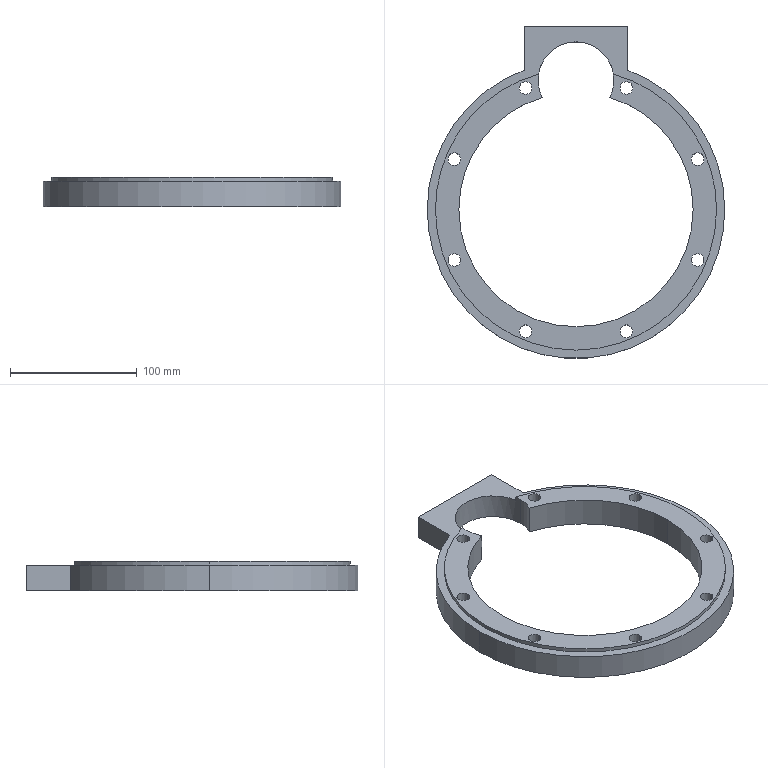Part | SolidWorks | features ICE 2, Cut 1, Extrusion 1, HoleWzd 1 | 1 solid | 34 faces | box 235 x 262.5 x 23 mm | volume 355148 mm3 | cylinder 28 | plane 6 | commonest cylinder face diameters 10 x16 60 x3 185 x3 222 x3 235 x3
STEP:
#1=CARTESIAN_POINT('',(44.799,96.083,23.));
#2=VERTEX_POINT('',#1);
#3=CARTESIAN_POINT('',(34.799,96.083,23.));
#4=VERTEX_POINT('',#3);
#5=CARTESIAN_POINT('',(39.799,96.083,23.));
#6=DIRECTION('',(0.,0.,-1.));
#7=DIRECTION('',(-1.,0.,0.));
#8=AXIS2_PLACEMENT_3D('',#5,#6,#7);
#9=CIRCLE('',#8,5.);
#10=EDGE_CURVE('',#2,#4,#9,.T.);
#11=ORIENTED_EDGE('',*,*,#10,.F.);
#12=CARTESIAN_POINT('',(44.799,96.083,0.));
#13=VERTEX_POINT('',#12);
#14=CARTESIAN_POINT('',(44.799,96.083,0.));
#15=DIRECTION('',(0.,0.,-1.));
#16=VECTOR('',#15,1000.);
#17=LINE('',#14,#16);
#18=EDGE_CURVE('',#2,#13,#17,.T.);
#19=ORIENTED_EDGE('',*,*,#18,.T.);
#20=CARTESIAN_POINT('',(34.799,96.083,0.));
#21=VERTEX_POINT('',#20);
#22=CARTESIAN_POINT('',(39.799,96.083,0.));
#23=DIRECTION('',(0.,0.,-1.));
#24=DIRECTION('',(-1.,0.,0.));
#25=AXIS2_PLACEMENT_3D('',#22,#23,#24);
#26=CIRCLE('',#25,5.);
#27=EDGE_CURVE('',#13,#21,#26,.T.);
#28=ORIENTED_EDGE('',*,*,#27,.T.);
#29=CARTESIAN_POINT('',(34.799,96.083,0.));
#30=DIRECTION('',(0.,0.,-1.));
#31=VECTOR('',#30,1000.);
#32=LINE('',#29,#31);
#33=EDGE_CURVE('',#4,#21,#32,.T.);
#34=ORIENTED_EDGE('',*,*,#33,.F.);
#35=EDGE_LOOP('',(#11,#19,#28,#34));
#36=FACE_OUTER_BOUND('',#35,.T.);
#37=CARTESIAN_POINT('',(39.799,96.083,0.));
#38=DIRECTION('',(0.,0.,-1.));
#39=DIRECTION('',(-1.,0.,0.));
#40=AXIS2_PLACEMENT_3D('',#37,#38,#39);
#41=CYLINDRICAL_SURFACE('',#40,5.);
#42=ADVANCED_FACE('',(#36),#41,.F.);
#43=CARTESIAN_POINT('',(101.083,39.799,23.));
#44=VERTEX_POINT('',#43);
#45=CARTESIAN_POINT('',(91.083,39.799,23.));
#46=VERTEX_POINT('',#45);
#47=CARTESIAN_POINT('',(96.083,39.799,23.));
#48=DIRECTION('',(0.,0.,-1.));
#49=DIRECTION('',(-1.,0.,0.));
#50=AXIS2_PLACEMENT_3D('',#47,#48,#49);
#51=CIRCLE('',#50,5.);
#52=EDGE_CURVE('',#44,#46,#51,.T.);
#53=ORIENTED_EDGE('',*,*,#52,.F.);
#54=CARTESIAN_POINT('',(101.083,39.799,0.));
#55=VERTEX_POINT('',#54);
#56=CARTESIAN_POINT('',(101.083,39.799,0.));
#57=DIRECTION('',(0.,0.,-1.));
#58=VECTOR('',#57,1000.);
#59=LINE('',#56,#58);
#60=EDGE_CURVE('',#44,#55,#59,.T.);
#61=ORIENTED_EDGE('',*,*,#60,.T.);
#62=CARTESIAN_POINT('',(91.083,39.799,0.));
#63=VERTEX_POINT('',#62);
#64=CARTESIAN_POINT('',(96.083,39.799,0.));
#65=DIRECTION('',(0.,0.,-1.));
#66=DIRECTION('',(-1.,0.,0.));
#67=AXIS2_PLACEMENT_3D('',#64,#65,#66);
#68=CIRCLE('',#67,5.);
#69=EDGE_CURVE('',#55,#63,#68,.T.);
#70=ORIENTED_EDGE('',*,*,#69,.T.);
#71=CARTESIAN_POINT('',(91.083,39.799,0.));
#72=DIRECTION('',(0.,0.,-1.));
#73=VECTOR('',#72,1000.);
#74=LINE('',#71,#73);
#75=EDGE_CURVE('',#46,#63,#74,.T.);
#76=ORIENTED_EDGE('',*,*,#75,.F.);
#77=EDGE_LOOP('',(#53,#61,#70,#76));
#78=FACE_OUTER_BOUND('',#77,.T.);
#79=CARTESIAN_POINT('',(96.083,39.799,0.));
#80=DIRECTION('',(0.,0.,-1.));
#81=DIRECTION('',(-1.,0.,0.));
#82=AXIS2_PLACEMENT_3D('',#79,#80,#81);
#83=CYLINDRICAL_SURFACE('',#82,5.);
#84=ADVANCED_FACE('',(#78),#83,.F.);
#85=CARTESIAN_POINT('',(101.083,-39.799,23.));
#86=VERTEX_POINT('',#85);
#87=CARTESIAN_POINT('',(91.083,-39.799,23.));
#88=VERTEX_POINT('',#87);
#89=CARTESIAN_POINT('',(96.083,-39.799,23.));
#90=DIRECTION('',(0.,0.,-1.));
#91=DIRECTION('',(-1.,0.,0.));
#92=AXIS2_PLACEMENT_3D('',#89,#90,#91);
#93=CIRCLE('',#92,5.);
#94=EDGE_CURVE('',#86,#88,#93,.T.);
#95=ORIENTED_EDGE('',*,*,#94,.F.);
#96=CARTESIAN_POINT('',(101.083,-39.799,0.));
#97=VERTEX_POINT('',#96);
#98=CARTESIAN_POINT('',(101.083,-39.799,0.));
#99=DIRECTION('',(0.,0.,-1.));
#100=VECTOR('',#99,1000.);
#101=LINE('',#98,#100);
#102=EDGE_CURVE('',#86,#97,#101,.T.);
#103=ORIENTED_EDGE('',*,*,#102,.T.);
#104=CARTESIAN_POINT('',(91.083,-39.799,0.));
#105=VERTEX_POINT('',#104);
#106=CARTESIAN_POINT('',(96.083,-39.799,0.));
#107=DIRECTION('',(0.,0.,-1.));
#108=DIRECTION('',(-1.,0.,0.));
#109=AXIS2_PLACEMENT_3D('',#106,#107,#108);
#110=CIRCLE('',#109,5.);
#111=EDGE_CURVE('',#97,#105,#110,.T.);
#112=ORIENTED_EDGE('',*,*,#111,.T.);
#113=CARTESIAN_POINT('',(91.083,-39.799,0.));
#114=DIRECTION('',(0.,0.,-1.));
#115=VECTOR('',#114,1000.);
#116=LINE('',#113,#115);
#117=EDGE_CURVE('',#88,#105,#116,.T.);
#118=ORIENTED_EDGE('',*,*,#117,.F.);
#119=EDGE_LOOP('',(#95,#103,#112,#118));
#120=FACE_OUTER_BOUND('',#119,.T.);
#121=CARTESIAN_POINT('',(96.083,-39.799,0.));
#122=DIRECTION('',(0.,0.,-1.));
#123=DIRECTION('',(-1.,0.,0.));
#124=AXIS2_PLACEMENT_3D('',#121,#122,#123);
#125=CYLINDRICAL_SURFACE('',#124,5.);
#126=ADVANCED_FACE('',(#120),#125,.F.);
#127=CARTESIAN_POINT('',(44.799,-96.083,23.));
#128=VERTEX_POINT('',#127);
#129=CARTESIAN_POINT('',(34.799,-96.083,23.));
#130=VERTEX_POINT('',#129);
#131=CARTESIAN_POINT('',(39.799,-96.083,23.));
#132=DIRECTION('',(0.,0.,-1.));
#133=DIRECTION('',(-1.,0.,0.));
#134=AXIS2_PLACEMENT_3D('',#131,#132,#133);
#135=CIRCLE('',#134,5.);
#136=EDGE_CURVE('',#128,#130,#135,.T.);
#137=ORIENTED_EDGE('',*,*,#136,.F.);
#138=CARTESIAN_POINT('',(44.799,-96.083,0.));
#139=VERTEX_POINT('',#138);
#140=CARTESIAN_POINT('',(44.799,-96.083,0.));
#141=DIRECTION('',(0.,0.,-1.));
#142=VECTOR('',#141,1000.);
#143=LINE('',#140,#142);
#144=EDGE_CURVE('',#128,#139,#143,.T.);
#145=ORIENTED_EDGE('',*,*,#144,.T.);
#146=CARTESIAN_POINT('',(34.799,-96.083,0.));
#147=VERTEX_POINT('',#146);
#148=CARTESIAN_POINT('',(39.799,-96.083,0.));
#149=DIRECTION('',(0.,0.,-1.));
#150=DIRECTION('',(-1.,0.,0.));
#151=AXIS2_PLACEMENT_3D('',#148,#149,#150);
#152=CIRCLE('',#151,5.);
#153=EDGE_CURVE('',#139,#147,#152,.T.);
#154=ORIENTED_EDGE('',*,*,#153,.T.);
#155=CARTESIAN_POINT('',(34.799,-96.083,0.));
#156=DIRECTION('',(0.,0.,-1.));
#157=VECTOR('',#156,1000.);
#158=LINE('',#155,#157);
#159=EDGE_CURVE('',#130,#147,#158,.T.);
#160=ORIENTED_EDGE('',*,*,#159,.F.);
#161=EDGE_LOOP('',(#137,#145,#154,#160));
#162=FACE_OUTER_BOUND('',#161,.T.);
#163=CARTESIAN_POINT('',(39.799,-96.083,0.));
#164=DIRECTION('',(0.,0.,-1.));
#165=DIRECTION('',(-1.,0.,0.));
#166=AXIS2_PLACEMENT_3D('',#163,#164,#165);
#167=CYLINDRICAL_SURFACE('',#166,5.);
#168=ADVANCED_FACE('',(#162),#167,.F.);
#169=CARTESIAN_POINT('',(-34.799,-96.083,23.));
#170=VERTEX_POINT('',#169);
#171=CARTESIAN_POINT('',(-44.799,-96.083,23.));
#172=VERTEX_POINT('',#171);
#173=CARTESIAN_POINT('',(-39.799,-96.083,23.));
#174=DIRECTION('',(0.,0.,-1.));
#175=DIRECTION('',(-1.,0.,0.));
#176=AXIS2_PLACEMENT_3D('',#173,#174,#175);
#177=CIRCLE('',#176,5.);
#178=EDGE_CURVE('',#170,#172,#177,.T.);
#179=ORIENTED_EDGE('',*,*,#178,.F.);
#180=CARTESIAN_POINT('',(-34.799,-96.083,0.));
#181=VERTEX_POINT('',#180);
#182=CARTESIAN_POINT('',(-34.799,-96.083,0.));
#183=DIRECTION('',(0.,0.,-1.));
#184=VECTOR('',#183,1000.);
#185=LINE('',#182,#184);
#186=EDGE_CURVE('',#170,#181,#185,.T.);
#187=ORIENTED_EDGE('',*,*,#186,.T.);
#188=CARTESIAN_POINT('',(-44.799,-96.083,0.));
#189=VERTEX_POINT('',#188);
#190=CARTESIAN_POINT('',(-39.799,-96.083,0.));
#191=DIRECTION('',(0.,0.,-1.));
#192=DIRECTION('',(-1.,0.,0.));
#193=AXIS2_PLACEMENT_3D('',#190,#191,#192);
#194=CIRCLE('',#193,5.);
#195=EDGE_CURVE('',#181,#189,#194,.T.);
#196=ORIENTED_EDGE('',*,*,#195,.T.);
#197=CARTESIAN_POINT('',(-44.799,-96.083,0.));
#198=DIRECTION('',(0.,0.,-1.));
#199=VECTOR('',#198,1000.);
#200=LINE('',#197,#199);
#201=EDGE_CURVE('',#172,#189,#200,.T.);
#202=ORIENTED_EDGE('',*,*,#201,.F.);
#203=EDGE_LOOP('',(#179,#187,#196,#202));
#204=FACE_OUTER_BOUND('',#203,.T.);
#205=CARTESIAN_POINT('',(-39.799,-96.083,0.));
#206=DIRECTION('',(0.,0.,-1.));
#207=DIRECTION('',(-1.,0.,0.));
#208=AXIS2_PLACEMENT_3D('',#205,#206,#207);
#209=CYLINDRICAL_SURFACE('',#208,5.);
#210=ADVANCED_FACE('',(#204),#209,.F.);
#211=CARTESIAN_POINT('',(-91.083,-39.799,23.));
#212=VERTEX_POINT('',#211);
#213=CARTESIAN_POINT('',(-101.083,-39.799,23.));
#214=VERTEX_POINT('',#213);
#215=CARTESIAN_POINT('',(-96.083,-39.799,23.));
#216=DIRECTION('',(0.,0.,-1.));
#217=DIRECTION('',(-1.,0.,0.));
#218=AXIS2_PLACEMENT_3D('',#215,#216,#217);
#219=CIRCLE('',#218,5.);
#220=EDGE_CURVE('',#212,#214,#219,.T.);
#221=ORIENTED_EDGE('',*,*,#220,.F.);
#222=CARTESIAN_POINT('',(-91.083,-39.799,0.));
#223=VERTEX_POINT('',#222);
#224=CARTESIAN_POINT('',(-91.083,-39.799,0.));
#225=DIRECTION('',(0.,0.,-1.));
#226=VECTOR('',#225,1000.);
#227=LINE('',#224,#226);
#228=EDGE_CURVE('',#212,#223,#227,.T.);
#229=ORIENTED_EDGE('',*,*,#228,.T.);
#230=CARTESIAN_POINT('',(-101.083,-39.799,0.));
#231=VERTEX_POINT('',#230);
#232=CARTESIAN_POINT('',(-96.083,-39.799,0.));
#233=DIRECTION('',(0.,0.,-1.));
#234=DIRECTION('',(-1.,0.,0.));
#235=AXIS2_PLACEMENT_3D('',#232,#233,#234);
#236=CIRCLE('',#235,5.);
#237=EDGE_CURVE('',#223,#231,#236,.T.);
#238=ORIENTED_EDGE('',*,*,#237,.T.);
#239=CARTESIAN_POINT('',(-101.083,-39.799,0.));
#240=DIRECTION('',(0.,0.,-1.));
#241=VECTOR('',#240,1000.);
#242=LINE('',#239,#241);
#243=EDGE_CURVE('',#214,#231,#242,.T.);
#244=ORIENTED_EDGE('',*,*,#243,.F.);
#245=EDGE_LOOP('',(#221,#229,#238,#244));
#246=FACE_OUTER_BOUND('',#245,.T.);
#247=CARTESIAN_POINT('',(-96.083,-39.799,0.));
#248=DIRECTION('',(0.,0.,-1.));
#249=DIRECTION('',(-1.,0.,0.));
#250=AXIS2_PLACEMENT_3D('',#247,#248,#249);
#251=CYLINDRICAL_SURFACE('',#250,5.);
#252=ADVANCED_FACE('',(#246),#251,.F.);
#253=CARTESIAN_POINT('',(-91.083,39.799,23.));
#254=VERTEX_POINT('',#253);
#255=CARTESIAN_POINT('',(-101.083,39.799,23.));
#256=VERTEX_POINT('',#255);
#257=CARTESIAN_POINT('',(-96.083,39.799,23.));
#258=DIRECTION('',(0.,0.,-1.));
#259=DIRECTION('',(-1.,0.,0.));
#260=AXIS2_PLACEMENT_3D('',#257,#258,#259);
#261=CIRCLE('',#260,5.);
#262=EDGE_CURVE('',#254,#256,#261,.T.);
#263=ORIENTED_EDGE('',*,*,#262,.F.);
#264=CARTESIAN_POINT('',(-91.083,39.799,0.));
#265=VERTEX_POINT('',#264);
#266=CARTESIAN_POINT('',(-91.083,39.799,0.));
#267=DIRECTION('',(0.,0.,-1.));
#268=VECTOR('',#267,1000.);
#269=LINE('',#266,#268);
#270=EDGE_CURVE('',#254,#265,#269,.T.);
#271=ORIENTED_EDGE('',*,*,#270,.T.);
#272=CARTESIAN_POINT('',(-101.083,39.799,0.));
#273=VERTEX_POINT('',#272);
#274=CARTESIAN_POINT('',(-96.083,39.799,0.));
#275=DIRECTION('',(0.,0.,-1.));
#276=DIRECTION('',(-1.,0.,0.));
#277=AXIS2_PLACEMENT_3D('',#274,#275,#276);
#278=CIRCLE('',#277,5.);
#279=EDGE_CURVE('',#265,#273,#278,.T.);
#280=ORIENTED_EDGE('',*,*,#279,.T.);
#281=CARTESIAN_POINT('',(-101.083,39.799,0.));
#282=DIRECTION('',(0.,0.,-1.));
#283=VECTOR('',#282,1000.);
#284=LINE('',#281,#283);
#285=EDGE_CURVE('',#256,#273,#284,.T.);
#286=ORIENTED_EDGE('',*,*,#285,.F.);
#287=EDGE_LOOP('',(#263,#271,#280,#286));
#288=FACE_OUTER_BOUND('',#287,.T.);
#289=CARTESIAN_POINT('',(-96.083,39.799,0.));
#290=DIRECTION('',(0.,0.,-1.));
#291=DIRECTION('',(-1.,0.,0.));
#292=AXIS2_PLACEMENT_3D('',#289,#290,#291);
#293=CYLINDRICAL_SURFACE('',#292,5.);
#294=ADVANCED_FACE('',(#288),#293,.F.);
#295=CARTESIAN_POINT('',(-34.799,96.083,23.));
#296=VERTEX_POINT('',#295);
#297=CARTESIAN_POINT('',(-44.799,96.083,23.));
#298=VERTEX_POINT('',#297);
#299=CARTESIAN_POINT('',(-39.799,96.083,23.));
#300=DIRECTION('',(0.,0.,-1.));
#301=DIRECTION('',(-1.,0.,0.));
#302=AXIS2_PLACEMENT_3D('',#299,#300,#301);
#303=CIRCLE('',#302,5.);
#304=EDGE_CURVE('',#296,#298,#303,.T.);
#305=ORIENTED_EDGE('',*,*,#304,.F.);
#306=CARTESIAN_POINT('',(-34.799,96.083,0.));
#307=VERTEX_POINT('',#306);
#308=CARTESIAN_POINT('',(-34.799,96.083,0.));
#309=DIRECTION('',(0.,0.,-1.));
#310=VECTOR('',#309,1000.);
#311=LINE('',#308,#310);
#312=EDGE_CURVE('',#296,#307,#311,.T.);
#313=ORIENTED_EDGE('',*,*,#312,.T.);
#314=CARTESIAN_POINT('',(-44.799,96.083,0.));
#315=VERTEX_POINT('',#314);
#316=CARTESIAN_POINT('',(-39.799,96.083,0.));
#317=DIRECTION('',(0.,0.,-1.));
#318=DIRECTION('',(-1.,0.,0.));
#319=AXIS2_PLACEMENT_3D('',#316,#317,#318);
#320=CIRCLE('',#319,5.);
#321=EDGE_CURVE('',#307,#315,#320,.T.);
#322=ORIENTED_EDGE('',*,*,#321,.T.);
#323=CARTESIAN_POINT('',(-44.799,96.083,0.));
#324=DIRECTION('',(0.,0.,-1.));
#325=VECTOR('',#324,1000.);
#326=LINE('',#323,#325);
#327=EDGE_CURVE('',#298,#315,#326,.T.);
#328=ORIENTED_EDGE('',*,*,#327,.F.);
#329=EDGE_LOOP('',(#305,#313,#322,#328));
#330=FACE_OUTER_BOUND('',#329,.T.);
#331=CARTESIAN_POINT('',(-39.799,96.083,0.));
#332=DIRECTION('',(0.,0.,-1.));
#333=DIRECTION('',(-1.,0.,0.));
#334=AXIS2_PLACEMENT_3D('',#331,#332,#333);
#335=CYLINDRICAL_SURFACE('',#334,5.);
#336=ADVANCED_FACE('',(#330),#335,.F.);
#337=CARTESIAN_POINT('',(30.,102.5,23.));
#338=VERTEX_POINT('',#337);
#339=CARTESIAN_POINT('',(26.584,88.598,23.));
#340=VERTEX_POINT('',#339);
#341=CARTESIAN_POINT('',(0.,102.5,23.));
#342=DIRECTION('',(0.,0.,-1.));
#343=DIRECTION('',(-1.,0.,0.));
#344=AXIS2_PLACEMENT_3D('',#341,#342,#343);
#345=CIRCLE('',#344,30.);
#346=EDGE_CURVE('',#338,#340,#345,.T.);
#347=ORIENTED_EDGE('',*,*,#346,.F.);
#348=CARTESIAN_POINT('',(30.,102.5,0.));
#349=VERTEX_POINT('',#348);
#350=CARTESIAN_POINT('',(30.,102.5,23.));
#351=DIRECTION('',(0.,0.,-1.));
#352=VECTOR('',#351,1000.);
#353=LINE('',#350,#352);
#354=EDGE_CURVE('',#338,#349,#353,.T.);
#355=ORIENTED_EDGE('',*,*,#354,.T.);
#356=CARTESIAN_POINT('',(26.584,88.598,0.));
#357=VERTEX_POINT('',#356);
#358=CARTESIAN_POINT('',(0.,102.5,0.));
#359=DIRECTION('',(0.,0.,-1.));
#360=DIRECTION('',(-1.,0.,0.));
#361=AXIS2_PLACEMENT_3D('',#358,#359,#360);
#362=CIRCLE('',#361,30.);
#363=EDGE_CURVE('',#349,#357,#362,.T.);
#364=ORIENTED_EDGE('',*,*,#363,.T.);
#365=CARTESIAN_POINT('',(26.584,88.598,11.5));
#366=DIRECTION('',(0.,0.,1.));
#367=VECTOR('',#366,1000.);
#368=LINE('',#365,#367);
#369=EDGE_CURVE('',#357,#340,#368,.T.);
#370=ORIENTED_EDGE('',*,*,#369,.T.);
#371=EDGE_LOOP('',(#347,#355,#364,#370));
#372=FACE_OUTER_BOUND('',#371,.T.);
#373=CARTESIAN_POINT('',(0.,102.5,23.));
#374=DIRECTION('',(0.,0.,-1.));
#375=DIRECTION('',(-1.,0.,0.));
#376=AXIS2_PLACEMENT_3D('',#373,#374,#375);
#377=CYLINDRICAL_SURFACE('',#376,30.);
#378=ADVANCED_FACE('',(#372),#377,.F.);
#379=ORIENTED_EDGE('',*,*,#354,.F.);
#380=CARTESIAN_POINT('',(29.666,106.962,23.));
#381=VERTEX_POINT('',#380);
#382=CARTESIAN_POINT('',(0.,102.5,23.));
#383=DIRECTION('',(0.,0.,-1.));
#384=DIRECTION('',(-1.,0.,0.));
#385=AXIS2_PLACEMENT_3D('',#382,#383,#384);
#386=CIRCLE('',#385,30.);
#387=EDGE_CURVE('',#381,#338,#386,.T.);
#388=ORIENTED_EDGE('',*,*,#387,.F.);
#389=CARTESIAN_POINT('',(29.666,106.962,20.));
#390=VERTEX_POINT('',#389);
#391=CARTESIAN_POINT('',(29.666,106.962,11.5));
#392=DIRECTION('',(0.,0.,1.));
#393=VECTOR('',#392,1000.);
#394=LINE('',#391,#393);
#395=EDGE_CURVE('',#390,#381,#394,.T.);
#396=ORIENTED_EDGE('',*,*,#395,.F.);
#397=CARTESIAN_POINT('',(-29.666,106.962,20.));
#398=VERTEX_POINT('',#397);
#399=CARTESIAN_POINT('',(0.,102.5,20.));
#400=DIRECTION('',(0.,0.,1.));
#401=DIRECTION('',(1.,0.,0.));
#402=AXIS2_PLACEMENT_3D('',#399,#400,#401);
#403=CIRCLE('',#402,30.);
#404=EDGE_CURVE('',#390,#398,#403,.T.);
#405=ORIENTED_EDGE('',*,*,#404,.T.);
#406=CARTESIAN_POINT('',(-29.666,106.962,23.));
#407=VERTEX_POINT('',#406);
#408=CARTESIAN_POINT('',(-29.666,106.962,11.5));
#409=DIRECTION('',(0.,0.,-1.));
#410=VECTOR('',#409,1000.);
#411=LINE('',#408,#410);
#412=EDGE_CURVE('',#407,#398,#411,.T.);
#413=ORIENTED_EDGE('',*,*,#412,.F.);
#414=CARTESIAN_POINT('',(-30.,102.5,23.));
#415=VERTEX_POINT('',#414);
#416=CARTESIAN_POINT('',(0.,102.5,23.));
#417=DIRECTION('',(0.,0.,-1.));
#418=DIRECTION('',(-1.,0.,0.));
#419=AXIS2_PLACEMENT_3D('',#416,#417,#418);
#420=CIRCLE('',#419,30.);
#421=EDGE_CURVE('',#415,#407,#420,.T.);
#422=ORIENTED_EDGE('',*,*,#421,.F.);
#423=CARTESIAN_POINT('',(-30.,102.5,0.));
#424=VERTEX_POINT('',#423);
#425=CARTESIAN_POINT('',(-30.,102.5,23.));
#426=DIRECTION('',(0.,0.,-1.));
#427=VECTOR('',#426,1000.);
#428=LINE('',#425,#427);
#429=EDGE_CURVE('',#415,#424,#428,.T.);
#430=ORIENTED_EDGE('',*,*,#429,.T.);
#431=CARTESIAN_POINT('',(0.,102.5,0.));
#432=DIRECTION('',(0.,0.,-1.));
#433=DIRECTION('',(-1.,0.,0.));
#434=AXIS2_PLACEMENT_3D('',#431,#432,#433);
#435=CIRCLE('',#434,30.);
#436=EDGE_CURVE('',#424,#349,#435,.T.);
#437=ORIENTED_EDGE('',*,*,#436,.T.);
#438=EDGE_LOOP('',(#379,#388,#396,#405,#413,#422,#430,#437));
#439=FACE_OUTER_BOUND('',#438,.T.);
#440=CARTESIAN_POINT('',(0.,102.5,23.));
#441=DIRECTION('',(0.,0.,-1.));
#442=DIRECTION('',(-1.,0.,0.));
#443=AXIS2_PLACEMENT_3D('',#440,#441,#442);
#444=CYLINDRICAL_SURFACE('',#443,30.);
#445=ADVANCED_FACE('',(#439),#444,.F.);
#446=CARTESIAN_POINT('',(111.,0.,23.));
#447=VERTEX_POINT('',#446);
#448=CARTESIAN_POINT('',(0.,0.,23.));
#449=DIRECTION('',(0.,0.,1.));
#450=DIRECTION('',(1.,0.,0.));
#451=AXIS2_PLACEMENT_3D('',#448,#449,#450);
#452=CIRCLE('',#451,111.);
#453=EDGE_CURVE('',#447,#381,#452,.T.);
#454=ORIENTED_EDGE('',*,*,#453,.F.);
#455=CARTESIAN_POINT('',(111.,0.,20.));
#456=VERTEX_POINT('',#455);
#457=CARTESIAN_POINT('',(111.,0.,23.));
#458=DIRECTION('',(0.,0.,-1.));
#459=VECTOR('',#458,1000.);
#460=LINE('',#457,#459);
#461=EDGE_CURVE('',#447,#456,#460,.T.);
#462=ORIENTED_EDGE('',*,*,#461,.T.);
#463=CARTESIAN_POINT('',(0.,0.,20.));
#464=DIRECTION('',(0.,0.,1.));
#465=DIRECTION('',(1.,0.,0.));
#466=AXIS2_PLACEMENT_3D('',#463,#464,#465);
#467=CIRCLE('',#466,111.);
#468=EDGE_CURVE('',#456,#390,#467,.T.);
#469=ORIENTED_EDGE('',*,*,#468,.T.);
#470=ORIENTED_EDGE('',*,*,#395,.T.);
#471=EDGE_LOOP('',(#454,#462,#469,#470));
#472=FACE_OUTER_BOUND('',#471,.T.);
#473=CARTESIAN_POINT('',(0.,0.,23.));
#474=DIRECTION('',(0.,0.,-1.));
#475=DIRECTION('',(-1.,0.,0.));
#476=AXIS2_PLACEMENT_3D('',#473,#474,#475);
#477=CYLINDRICAL_SURFACE('',#476,111.);
#478=ADVANCED_FACE('',(#472),#477,.T.);
#479=ORIENTED_EDGE('',*,*,#461,.F.);
#480=CARTESIAN_POINT('',(-111.,0.,23.));
#481=VERTEX_POINT('',#480);
#482=CARTESIAN_POINT('',(0.,0.,23.));
#483=DIRECTION('',(0.,0.,1.));
#484=DIRECTION('',(1.,0.,0.));
#485=AXIS2_PLACEMENT_3D('',#482,#483,#484);
#486=CIRCLE('',#485,111.);
#487=EDGE_CURVE('',#481,#447,#486,.T.);
#488=ORIENTED_EDGE('',*,*,#487,.F.);
#489=CARTESIAN_POINT('',(-111.,0.,20.));
#490=VERTEX_POINT('',#489);
#491=CARTESIAN_POINT('',(-111.,0.,23.));
#492=DIRECTION('',(0.,0.,-1.));
#493=VECTOR('',#492,1000.);
#494=LINE('',#491,#493);
#495=EDGE_CURVE('',#481,#490,#494,.T.);
#496=ORIENTED_EDGE('',*,*,#495,.T.);
#497=CARTESIAN_POINT('',(0.,0.,20.));
#498=DIRECTION('',(0.,0.,1.));
#499=DIRECTION('',(1.,0.,0.));
#500=AXIS2_PLACEMENT_3D('',#497,#498,#499);
#501=CIRCLE('',#500,111.);
#502=EDGE_CURVE('',#490,#456,#501,.T.);
#503=ORIENTED_EDGE('',*,*,#502,.T.);
#504=EDGE_LOOP('',(#479,#488,#496,#503));
#505=FACE_OUTER_BOUND('',#504,.T.);
#506=CARTESIAN_POINT('',(0.,0.,23.));
#507=DIRECTION('',(0.,0.,-1.));
#508=DIRECTION('',(-1.,0.,0.));
#509=AXIS2_PLACEMENT_3D('',#506,#507,#508);
#510=CYLINDRICAL_SURFACE('',#509,111.);
#511=ADVANCED_FACE('',(#505),#510,.T.);
#512=CARTESIAN_POINT('',(-92.5,0.,23.));
#513=VERTEX_POINT('',#512);
#514=CARTESIAN_POINT('',(92.5,0.,23.));
#515=VERTEX_POINT('',#514);
#516=CARTESIAN_POINT('',(0.,0.,23.));
#517=DIRECTION('',(0.,0.,1.));
#518=DIRECTION('',(1.,0.,0.));
#519=AXIS2_PLACEMENT_3D('',#516,#517,#518);
#520=CIRCLE('',#519,92.5);
#521=EDGE_CURVE('',#513,#515,#520,.T.);
#522=ORIENTED_EDGE('',*,*,#521,.T.);
#523=CARTESIAN_POINT('',(92.5,0.,0.));
#524=VERTEX_POINT('',#523);
#525=CARTESIAN_POINT('',(92.5,0.,20.));
#526=DIRECTION('',(0.,0.,-1.));
#527=VECTOR('',#526,1000.);
#528=LINE('',#525,#527);
#529=EDGE_CURVE('',#515,#524,#528,.T.);
#530=ORIENTED_EDGE('',*,*,#529,.T.);
#531=CARTESIAN_POINT('',(-92.5,0.,0.));
#532=VERTEX_POINT('',#531);
#533=CARTESIAN_POINT('',(0.,0.,0.));
#534=DIRECTION('',(0.,0.,1.));
#535=DIRECTION('',(1.,0.,0.));
#536=AXIS2_PLACEMENT_3D('',#533,#534,#535);
#537=CIRCLE('',#536,92.5);
#538=EDGE_CURVE('',#532,#524,#537,.T.);
#539=ORIENTED_EDGE('',*,*,#538,.F.);
#540=CARTESIAN_POINT('',(-92.5,0.,20.));
#541=DIRECTION('',(0.,0.,-1.));
#542=VECTOR('',#541,1000.);
#543=LINE('',#540,#542);
#544=EDGE_CURVE('',#513,#532,#543,.T.);
#545=ORIENTED_EDGE('',*,*,#544,.F.);
#546=EDGE_LOOP('',(#522,#530,#539,#545));
#547=FACE_OUTER_BOUND('',#546,.T.);
#548=CARTESIAN_POINT('',(0.,0.,20.));
#549=DIRECTION('',(0.,0.,-1.));
#550=DIRECTION('',(-1.,0.,0.));
#551=AXIS2_PLACEMENT_3D('',#548,#549,#550);
#552=CYLINDRICAL_SURFACE('',#551,92.5);
#553=ADVANCED_FACE('',(#547),#552,.F.);
#554=CARTESIAN_POINT('',(-26.584,88.598,23.));
#555=VERTEX_POINT('',#554);
#556=CARTESIAN_POINT('',(0.,0.,23.));
#557=DIRECTION('',(0.,0.,1.));
#558=DIRECTION('',(1.,0.,0.));
#559=AXIS2_PLACEMENT_3D('',#556,#557,#558);
#560=CIRCLE('',#559,92.5);
#561=EDGE_CURVE('',#555,#513,#560,.T.);
#562=ORIENTED_EDGE('',*,*,#561,.T.);
#563=ORIENTED_EDGE('',*,*,#544,.T.);
#564=CARTESIAN_POINT('',(-26.584,88.598,0.));
#565=VERTEX_POINT('',#564);
#566=CARTESIAN_POINT('',(0.,0.,0.));
#567=DIRECTION('',(0.,0.,1.));
#568=DIRECTION('',(1.,0.,0.));
#569=AXIS2_PLACEMENT_3D('',#566,#567,#568);
#570=CIRCLE('',#569,92.5);
#571=EDGE_CURVE('',#565,#532,#570,.T.);
#572=ORIENTED_EDGE('',*,*,#571,.F.);
#573=CARTESIAN_POINT('',(-26.584,88.598,11.5));
#574=DIRECTION('',(0.,0.,-1.));
#575=VECTOR('',#574,1000.);
#576=LINE('',#573,#575);
#577=EDGE_CURVE('',#555,#565,#576,.T.);
#578=ORIENTED_EDGE('',*,*,#577,.F.);
#579=EDGE_LOOP('',(#562,#563,#572,#578));
#580=FACE_OUTER_BOUND('',#579,.T.);
#581=CARTESIAN_POINT('',(0.,0.,20.));
#582=DIRECTION('',(0.,0.,-1.));
#583=DIRECTION('',(-1.,0.,0.));
#584=AXIS2_PLACEMENT_3D('',#581,#582,#583);
#585=CYLINDRICAL_SURFACE('',#584,92.5);
#586=ADVANCED_FACE('',(#580),#585,.F.);
#587=CARTESIAN_POINT('',(117.5,0.,20.));
#588=VERTEX_POINT('',#587);
#589=CARTESIAN_POINT('',(41.,110.115,20.));
#590=VERTEX_POINT('',#589);
#591=CARTESIAN_POINT('',(0.,0.,20.));
#592=DIRECTION('',(0.,0.,1.));
#593=DIRECTION('',(1.,0.,0.));
#594=AXIS2_PLACEMENT_3D('',#591,#592,#593);
#595=CIRCLE('',#594,117.5);
#596=EDGE_CURVE('',#588,#590,#595,.T.);
#597=ORIENTED_EDGE('',*,*,#596,.F.);
#598=CARTESIAN_POINT('',(117.5,0.,0.));
#599=VERTEX_POINT('',#598);
#600=CARTESIAN_POINT('',(117.5,0.,20.));
#601=DIRECTION('',(0.,0.,-1.));
#602=VECTOR('',#601,1000.);
#603=LINE('',#600,#602);
#604=EDGE_CURVE('',#588,#599,#603,.T.);
#605=ORIENTED_EDGE('',*,*,#604,.T.);
#606=CARTESIAN_POINT('',(41.,110.115,0.));
#607=VERTEX_POINT('',#606);
#608=CARTESIAN_POINT('',(0.,0.,0.));
#609=DIRECTION('',(0.,0.,1.));
#610=DIRECTION('',(1.,0.,0.));
#611=AXIS2_PLACEMENT_3D('',#608,#609,#610);
#612=CIRCLE('',#611,117.5);
#613=EDGE_CURVE('',#599,#607,#612,.T.);
#614=ORIENTED_EDGE('',*,*,#613,.T.);
#615=CARTESIAN_POINT('',(41.,110.115,20.));
#616=DIRECTION('',(0.,0.,1.));
#617=VECTOR('',#616,1000.);
#618=LINE('',#615,#617);
#619=EDGE_CURVE('',#607,#590,#618,.T.);
#620=ORIENTED_EDGE('',*,*,#619,.T.);
#621=EDGE_LOOP('',(#597,#605,#614,#620));
#622=FACE_OUTER_BOUND('',#621,.T.);
#623=CARTESIAN_POINT('',(0.,0.,20.));
#624=DIRECTION('',(0.,0.,-1.));
#625=DIRECTION('',(-1.,0.,0.));
#626=AXIS2_PLACEMENT_3D('',#623,#624,#625);
#627=CYLINDRICAL_SURFACE('',#626,117.5);
#628=ADVANCED_FACE('',(#622),#627,.T.);
#629=ORIENTED_EDGE('',*,*,#604,.F.);
#630=CARTESIAN_POINT('',(-117.5,0.,20.));
#631=VERTEX_POINT('',#630);
#632=CARTESIAN_POINT('',(0.,0.,20.));
#633=DIRECTION('',(0.,0.,1.));
#634=DIRECTION('',(1.,0.,0.));
#635=AXIS2_PLACEMENT_3D('',#632,#633,#634);
#636=CIRCLE('',#635,117.5);
#637=EDGE_CURVE('',#631,#588,#636,.T.);
#638=ORIENTED_EDGE('',*,*,#637,.F.);
#639=CARTESIAN_POINT('',(-117.5,0.,0.));
#640=VERTEX_POINT('',#639);
#641=CARTESIAN_POINT('',(-117.5,0.,20.));
#642=DIRECTION('',(0.,0.,-1.));
#643=VECTOR('',#642,1000.);
#644=LINE('',#641,#643);
#645=EDGE_CURVE('',#631,#640,#644,.T.);
#646=ORIENTED_EDGE('',*,*,#645,.T.);
#647=CARTESIAN_POINT('',(0.,0.,0.));
#648=DIRECTION('',(0.,0.,1.));
#649=DIRECTION('',(1.,0.,0.));
#650=AXIS2_PLACEMENT_3D('',#647,#648,#649);
#651=CIRCLE('',#650,117.5);
#652=EDGE_CURVE('',#640,#599,#651,.T.);
#653=ORIENTED_EDGE('',*,*,#652,.T.);
#654=EDGE_LOOP('',(#629,#638,#646,#653));
#655=FACE_OUTER_BOUND('',#654,.T.);
#656=CARTESIAN_POINT('',(0.,0.,20.));
#657=DIRECTION('',(0.,0.,-1.));
#658=DIRECTION('',(-1.,0.,0.));
#659=AXIS2_PLACEMENT_3D('',#656,#657,#658);
#660=CYLINDRICAL_SURFACE('',#659,117.5);
#661=ADVANCED_FACE('',(#655),#660,.T.);
#662=ORIENTED_EDGE('',*,*,#404,.F.);
#663=ORIENTED_EDGE('',*,*,#468,.F.);
#664=ORIENTED_EDGE('',*,*,#502,.F.);
#665=CARTESIAN_POINT('',(0.,0.,20.));
#666=DIRECTION('',(0.,0.,1.));
#667=DIRECTION('',(1.,0.,0.));
#668=AXIS2_PLACEMENT_3D('',#665,#666,#667);
#669=CIRCLE('',#668,111.);
#670=EDGE_CURVE('',#398,#490,#669,.T.);
#671=ORIENTED_EDGE('',*,*,#670,.F.);
#672=EDGE_LOOP('',(#662,#663,#664,#671));
#673=FACE_BOUND('',#672,.T.);
#674=CARTESIAN_POINT('',(-41.,110.115,20.));
#675=VERTEX_POINT('',#674);
#676=CARTESIAN_POINT('',(0.,0.,20.));
#677=DIRECTION('',(0.,0.,1.));
#678=DIRECTION('',(1.,0.,0.));
#679=AXIS2_PLACEMENT_3D('',#676,#677,#678);
#680=CIRCLE('',#679,117.5);
#681=EDGE_CURVE('',#675,#631,#680,.T.);
#682=ORIENTED_EDGE('',*,*,#681,.T.);
#683=ORIENTED_EDGE('',*,*,#637,.T.);
#684=ORIENTED_EDGE('',*,*,#596,.T.);
#685=CARTESIAN_POINT('',(41.,145.,20.));
#686=VERTEX_POINT('',#685);
#687=CARTESIAN_POINT('',(41.,92.5,20.));
#688=DIRECTION('',(0.,1.,0.));
#689=VECTOR('',#688,1000.);
#690=LINE('',#687,#689);
#691=EDGE_CURVE('',#590,#686,#690,.T.);
#692=ORIENTED_EDGE('',*,*,#691,.T.);
#693=CARTESIAN_POINT('',(-41.,145.,20.));
#694=VERTEX_POINT('',#693);
#695=CARTESIAN_POINT('',(-41.,145.,20.));
#696=DIRECTION('',(-1.,0.,0.));
#697=VECTOR('',#696,1000.);
#698=LINE('',#695,#697);
#699=EDGE_CURVE('',#686,#694,#698,.T.);
#700=ORIENTED_EDGE('',*,*,#699,.T.);
#701=CARTESIAN_POINT('',(-41.,92.5,20.));
#702=DIRECTION('',(0.,-1.,0.));
#703=VECTOR('',#702,1000.);
#704=LINE('',#701,#703);
#705=EDGE_CURVE('',#694,#675,#704,.T.);
#706=ORIENTED_EDGE('',*,*,#705,.T.);
#707=EDGE_LOOP('',(#682,#683,#684,#692,#700,#706));
#708=FACE_OUTER_BOUND('',#707,.T.);
#709=CARTESIAN_POINT('',(0.,0.,20.));
#710=DIRECTION('',(0.,0.,1.));
#711=DIRECTION('',(1.,0.,0.));
#712=AXIS2_PLACEMENT_3D('',#709,#710,#711);
#713=PLANE('',#712);
#714=ADVANCED_FACE('',(#673,#708),#713,.T.);
#715=CARTESIAN_POINT('',(39.799,96.083,0.));
#716=DIRECTION('',(0.,0.,-1.));
#717=DIRECTION('',(-1.,0.,0.));
#718=AXIS2_PLACEMENT_3D('',#715,#716,#717);
#719=CIRCLE('',#718,5.);
#720=EDGE_CURVE('',#21,#13,#719,.T.);
#721=ORIENTED_EDGE('',*,*,#720,.F.);
#722=ORIENTED_EDGE('',*,*,#27,.F.);
#723=EDGE_LOOP('',(#721,#722));
#724=FACE_BOUND('',#723,.T.);
#725=CARTESIAN_POINT('',(96.083,39.799,0.));
#726=DIRECTION('',(0.,0.,-1.));
#727=DIRECTION('',(-1.,0.,0.));
#728=AXIS2_PLACEMENT_3D('',#725,#726,#727);
#729=CIRCLE('',#728,5.);
#730=EDGE_CURVE('',#63,#55,#729,.T.);
#731=ORIENTED_EDGE('',*,*,#730,.F.);
#732=ORIENTED_EDGE('',*,*,#69,.F.);
#733=EDGE_LOOP('',(#731,#732));
#734=FACE_BOUND('',#733,.T.);
#735=CARTESIAN_POINT('',(96.083,-39.799,0.));
#736=DIRECTION('',(0.,0.,-1.));
#737=DIRECTION('',(-1.,0.,0.));
#738=AXIS2_PLACEMENT_3D('',#735,#736,#737);
#739=CIRCLE('',#738,5.);
#740=EDGE_CURVE('',#105,#97,#739,.T.);
#741=ORIENTED_EDGE('',*,*,#740,.F.);
#742=ORIENTED_EDGE('',*,*,#111,.F.);
#743=EDGE_LOOP('',(#741,#742));
#744=FACE_BOUND('',#743,.T.);
#745=CARTESIAN_POINT('',(39.799,-96.083,0.));
#746=DIRECTION('',(0.,0.,-1.));
#747=DIRECTION('',(-1.,0.,0.));
#748=AXIS2_PLACEMENT_3D('',#745,#746,#747);
#749=CIRCLE('',#748,5.);
#750=EDGE_CURVE('',#147,#139,#749,.T.);
#751=ORIENTED_EDGE('',*,*,#750,.F.);
#752=ORIENTED_EDGE('',*,*,#153,.F.);
#753=EDGE_LOOP('',(#751,#752));
#754=FACE_BOUND('',#753,.T.);
#755=CARTESIAN_POINT('',(-39.799,-96.083,0.));
#756=DIRECTION('',(0.,0.,-1.));
#757=DIRECTION('',(-1.,0.,0.));
#758=AXIS2_PLACEMENT_3D('',#755,#756,#757);
#759=CIRCLE('',#758,5.);
#760=EDGE_CURVE('',#189,#181,#759,.T.);
#761=ORIENTED_EDGE('',*,*,#760,.F.);
#762=ORIENTED_EDGE('',*,*,#195,.F.);
#763=EDGE_LOOP('',(#761,#762));
#764=FACE_BOUND('',#763,.T.);
#765=CARTESIAN_POINT('',(-96.083,-39.799,0.));
#766=DIRECTION('',(0.,0.,-1.));
#767=DIRECTION('',(-1.,0.,0.));
#768=AXIS2_PLACEMENT_3D('',#765,#766,#767);
#769=CIRCLE('',#768,5.);
#770=EDGE_CURVE('',#231,#223,#769,.T.);
#771=ORIENTED_EDGE('',*,*,#770,.F.);
#772=ORIENTED_EDGE('',*,*,#237,.F.);
#773=EDGE_LOOP('',(#771,#772));
#774=FACE_BOUND('',#773,.T.);
#775=CARTESIAN_POINT('',(-96.083,39.799,0.));
#776=DIRECTION('',(0.,0.,-1.));
#777=DIRECTION('',(-1.,0.,0.));
#778=AXIS2_PLACEMENT_3D('',#775,#776,#777);
#779=CIRCLE('',#778,5.);
#780=EDGE_CURVE('',#273,#265,#779,.T.);
#781=ORIENTED_EDGE('',*,*,#780,.F.);
#782=ORIENTED_EDGE('',*,*,#279,.F.);
#783=EDGE_LOOP('',(#781,#782));
#784=FACE_BOUND('',#783,.T.);
#785=CARTESIAN_POINT('',(-39.799,96.083,0.));
#786=DIRECTION('',(0.,0.,-1.));
#787=DIRECTION('',(-1.,0.,0.));
#788=AXIS2_PLACEMENT_3D('',#785,#786,#787);
#789=CIRCLE('',#788,5.);
#790=EDGE_CURVE('',#315,#307,#789,.T.);
#791=ORIENTED_EDGE('',*,*,#790,.F.);
#792=ORIENTED_EDGE('',*,*,#321,.F.);
#793=EDGE_LOOP('',(#791,#792));
#794=FACE_BOUND('',#793,.T.);
#795=CARTESIAN_POINT('',(41.,145.,0.));
#796=VERTEX_POINT('',#795);
#797=CARTESIAN_POINT('',(41.,92.5,0.));
#798=DIRECTION('',(0.,1.,0.));
#799=VECTOR('',#798,1000.);
#800=LINE('',#797,#799);
#801=EDGE_CURVE('',#607,#796,#800,.T.);
#802=ORIENTED_EDGE('',*,*,#801,.F.);
#803=ORIENTED_EDGE('',*,*,#613,.F.);
#804=ORIENTED_EDGE('',*,*,#652,.F.);
#805=CARTESIAN_POINT('',(-41.,110.115,0.));
#806=VERTEX_POINT('',#805);
#807=CARTESIAN_POINT('',(0.,0.,0.));
#808=DIRECTION('',(0.,0.,1.));
#809=DIRECTION('',(1.,0.,0.));
#810=AXIS2_PLACEMENT_3D('',#807,#808,#809);
#811=CIRCLE('',#810,117.5);
#812=EDGE_CURVE('',#806,#640,#811,.T.);
#813=ORIENTED_EDGE('',*,*,#812,.F.);
#814=CARTESIAN_POINT('',(-41.,145.,0.));
#815=VERTEX_POINT('',#814);
#816=CARTESIAN_POINT('',(-41.,92.5,0.));
#817=DIRECTION('',(0.,-1.,0.));
#818=VECTOR('',#817,1000.);
#819=LINE('',#816,#818);
#820=EDGE_CURVE('',#815,#806,#819,.T.);
#821=ORIENTED_EDGE('',*,*,#820,.F.);
#822=CARTESIAN_POINT('',(-41.,145.,0.));
#823=DIRECTION('',(-1.,0.,0.));
#824=VECTOR('',#823,1000.);
#825=LINE('',#822,#824);
#826=EDGE_CURVE('',#796,#815,#825,.T.);
#827=ORIENTED_EDGE('',*,*,#826,.F.);
#828=EDGE_LOOP('',(#802,#803,#804,#813,#821,#827));
#829=FACE_OUTER_BOUND('',#828,.T.);
#830=ORIENTED_EDGE('',*,*,#571,.T.);
#831=ORIENTED_EDGE('',*,*,#538,.T.);
#832=CARTESIAN_POINT('',(0.,0.,0.));
#833=DIRECTION('',(0.,0.,1.));
#834=DIRECTION('',(1.,0.,0.));
#835=AXIS2_PLACEMENT_3D('',#832,#833,#834);
#836=CIRCLE('',#835,92.5);
#837=EDGE_CURVE('',#524,#357,#836,.T.);
#838=ORIENTED_EDGE('',*,*,#837,.T.);
#839=ORIENTED_EDGE('',*,*,#363,.F.);
#840=ORIENTED_EDGE('',*,*,#436,.F.);
#841=CARTESIAN_POINT('',(0.,102.5,0.));
#842=DIRECTION('',(0.,0.,-1.));
#843=DIRECTION('',(-1.,0.,0.));
#844=AXIS2_PLACEMENT_3D('',#841,#842,#843);
#845=CIRCLE('',#844,30.);
#846=EDGE_CURVE('',#565,#424,#845,.T.);
#847=ORIENTED_EDGE('',*,*,#846,.F.);
#848=EDGE_LOOP('',(#830,#831,#838,#839,#840,#847));
#849=FACE_BOUND('',#848,.T.);
#850=CARTESIAN_POINT('',(0.,0.,0.));
#851=DIRECTION('',(0.,0.,1.));
#852=DIRECTION('',(1.,0.,0.));
#853=AXIS2_PLACEMENT_3D('',#850,#851,#852);
#854=PLANE('',#853);
#855=ADVANCED_FACE('',(#724,#734,#744,#754,#764,#774,#784,#794,#829,#849),#854,.F.);
#856=ORIENTED_EDGE('',*,*,#645,.F.);
#857=ORIENTED_EDGE('',*,*,#681,.F.);
#858=CARTESIAN_POINT('',(-41.,110.115,20.));
#859=DIRECTION('',(0.,0.,-1.));
#860=VECTOR('',#859,1000.);
#861=LINE('',#858,#860);
#862=EDGE_CURVE('',#675,#806,#861,.T.);
#863=ORIENTED_EDGE('',*,*,#862,.T.);
#864=ORIENTED_EDGE('',*,*,#812,.T.);
#865=EDGE_LOOP('',(#856,#857,#863,#864));
#866=FACE_OUTER_BOUND('',#865,.T.);
#867=CARTESIAN_POINT('',(0.,0.,20.));
#868=DIRECTION('',(0.,0.,-1.));
#869=DIRECTION('',(-1.,0.,0.));
#870=AXIS2_PLACEMENT_3D('',#867,#868,#869);
#871=CYLINDRICAL_SURFACE('',#870,117.5);
#872=ADVANCED_FACE('',(#866),#871,.T.);
#873=ORIENTED_EDGE('',*,*,#529,.F.);
#874=CARTESIAN_POINT('',(0.,0.,23.));
#875=DIRECTION('',(0.,0.,1.));
#876=DIRECTION('',(1.,0.,0.));
#877=AXIS2_PLACEMENT_3D('',#874,#875,#876);
#878=CIRCLE('',#877,92.5);
#879=EDGE_CURVE('',#515,#340,#878,.T.);
#880=ORIENTED_EDGE('',*,*,#879,.T.);
#881=ORIENTED_EDGE('',*,*,#369,.F.);
#882=ORIENTED_EDGE('',*,*,#837,.F.);
#883=EDGE_LOOP('',(#873,#880,#881,#882));
#884=FACE_OUTER_BOUND('',#883,.T.);
#885=CARTESIAN_POINT('',(0.,0.,20.));
#886=DIRECTION('',(0.,0.,-1.));
#887=DIRECTION('',(-1.,0.,0.));
#888=AXIS2_PLACEMENT_3D('',#885,#886,#887);
#889=CYLINDRICAL_SURFACE('',#888,92.5);
#890=ADVANCED_FACE('',(#884),#889,.F.);
#891=ORIENTED_EDGE('',*,*,#619,.F.);
#892=ORIENTED_EDGE('',*,*,#801,.T.);
#893=CARTESIAN_POINT('',(41.,145.,0.));
#894=DIRECTION('',(0.,0.,1.));
#895=VECTOR('',#894,1000.);
#896=LINE('',#893,#895);
#897=EDGE_CURVE('',#796,#686,#896,.T.);
#898=ORIENTED_EDGE('',*,*,#897,.T.);
#899=ORIENTED_EDGE('',*,*,#691,.F.);
#900=EDGE_LOOP('',(#891,#892,#898,#899));
#901=FACE_OUTER_BOUND('',#900,.T.);
#902=CARTESIAN_POINT('',(41.,92.5,0.));
#903=DIRECTION('',(1.,0.,0.));
#904=DIRECTION('',(0.,0.,-1.));
#905=AXIS2_PLACEMENT_3D('',#902,#903,#904);
#906=PLANE('',#905);
#907=ADVANCED_FACE('',(#901),#906,.T.);
#908=ORIENTED_EDGE('',*,*,#862,.F.);
#909=ORIENTED_EDGE('',*,*,#705,.F.);
#910=CARTESIAN_POINT('',(-41.,145.,0.));
#911=DIRECTION('',(0.,0.,1.));
#912=VECTOR('',#911,1000.);
#913=LINE('',#910,#912);
#914=EDGE_CURVE('',#815,#694,#913,.T.);
#915=ORIENTED_EDGE('',*,*,#914,.F.);
#916=ORIENTED_EDGE('',*,*,#820,.T.);
#917=EDGE_LOOP('',(#908,#909,#915,#916));
#918=FACE_OUTER_BOUND('',#917,.T.);
#919=CARTESIAN_POINT('',(-41.,92.5,0.));
#920=DIRECTION('',(-1.,0.,0.));
#921=DIRECTION('',(0.,0.,1.));
#922=AXIS2_PLACEMENT_3D('',#919,#920,#921);
#923=PLANE('',#922);
#924=ADVANCED_FACE('',(#918),#923,.T.);
#925=ORIENTED_EDGE('',*,*,#699,.F.);
#926=ORIENTED_EDGE('',*,*,#897,.F.);
#927=ORIENTED_EDGE('',*,*,#826,.T.);
#928=ORIENTED_EDGE('',*,*,#914,.T.);
#929=EDGE_LOOP('',(#925,#926,#927,#928));
#930=FACE_OUTER_BOUND('',#929,.T.);
#931=CARTESIAN_POINT('',(-41.,145.,0.));
#932=DIRECTION('',(0.,1.,0.));
#933=DIRECTION('',(0.,0.,1.));
#934=AXIS2_PLACEMENT_3D('',#931,#932,#933);
#935=PLANE('',#934);
#936=ADVANCED_FACE('',(#930),#935,.T.);
#937=CARTESIAN_POINT('',(39.799,96.083,23.));
#938=DIRECTION('',(0.,0.,-1.));
#939=DIRECTION('',(-1.,0.,0.));
#940=AXIS2_PLACEMENT_3D('',#937,#938,#939);
#941=CIRCLE('',#940,5.);
#942=EDGE_CURVE('',#4,#2,#941,.T.);
#943=ORIENTED_EDGE('',*,*,#942,.T.);
#944=ORIENTED_EDGE('',*,*,#10,.T.);
#945=EDGE_LOOP('',(#943,#944));
#946=FACE_BOUND('',#945,.T.);
#947=CARTESIAN_POINT('',(96.083,39.799,23.));
#948=DIRECTION('',(0.,0.,-1.));
#949=DIRECTION('',(-1.,0.,0.));
#950=AXIS2_PLACEMENT_3D('',#947,#948,#949);
#951=CIRCLE('',#950,5.);
#952=EDGE_CURVE('',#46,#44,#951,.T.);
#953=ORIENTED_EDGE('',*,*,#952,.T.);
#954=ORIENTED_EDGE('',*,*,#52,.T.);
#955=EDGE_LOOP('',(#953,#954));
#956=FACE_BOUND('',#955,.T.);
#957=CARTESIAN_POINT('',(96.083,-39.799,23.));
#958=DIRECTION('',(0.,0.,-1.));
#959=DIRECTION('',(-1.,0.,0.));
#960=AXIS2_PLACEMENT_3D('',#957,#958,#959);
#961=CIRCLE('',#960,5.);
#962=EDGE_CURVE('',#88,#86,#961,.T.);
#963=ORIENTED_EDGE('',*,*,#962,.T.);
#964=ORIENTED_EDGE('',*,*,#94,.T.);
#965=EDGE_LOOP('',(#963,#964));
#966=FACE_BOUND('',#965,.T.);
#967=CARTESIAN_POINT('',(39.799,-96.083,23.));
#968=DIRECTION('',(0.,0.,-1.));
#969=DIRECTION('',(-1.,0.,0.));
#970=AXIS2_PLACEMENT_3D('',#967,#968,#969);
#971=CIRCLE('',#970,5.);
#972=EDGE_CURVE('',#130,#128,#971,.T.);
#973=ORIENTED_EDGE('',*,*,#972,.T.);
#974=ORIENTED_EDGE('',*,*,#136,.T.);
#975=EDGE_LOOP('',(#973,#974));
#976=FACE_BOUND('',#975,.T.);
#977=CARTESIAN_POINT('',(-39.799,-96.083,23.));
#978=DIRECTION('',(0.,0.,-1.));
#979=DIRECTION('',(-1.,0.,0.));
#980=AXIS2_PLACEMENT_3D('',#977,#978,#979);
#981=CIRCLE('',#980,5.);
#982=EDGE_CURVE('',#172,#170,#981,.T.);
#983=ORIENTED_EDGE('',*,*,#982,.T.);
#984=ORIENTED_EDGE('',*,*,#178,.T.);
#985=EDGE_LOOP('',(#983,#984));
#986=FACE_BOUND('',#985,.T.);
#987=CARTESIAN_POINT('',(-96.083,-39.799,23.));
#988=DIRECTION('',(0.,0.,-1.));
#989=DIRECTION('',(-1.,0.,0.));
#990=AXIS2_PLACEMENT_3D('',#987,#988,#989);
#991=CIRCLE('',#990,5.);
#992=EDGE_CURVE('',#214,#212,#991,.T.);
#993=ORIENTED_EDGE('',*,*,#992,.T.);
#994=ORIENTED_EDGE('',*,*,#220,.T.);
#995=EDGE_LOOP('',(#993,#994));
#996=FACE_BOUND('',#995,.T.);
#997=CARTESIAN_POINT('',(-96.083,39.799,23.));
#998=DIRECTION('',(0.,0.,-1.));
#999=DIRECTION('',(-1.,0.,0.));
#1000=AXIS2_PLACEMENT_3D('',#997,#998,#999);
#1001=CIRCLE('',#1000,5.);
#1002=EDGE_CURVE('',#256,#254,#1001,.T.);
#1003=ORIENTED_EDGE('',*,*,#1002,.T.);
#1004=ORIENTED_EDGE('',*,*,#262,.T.);
#1005=EDGE_LOOP('',(#1003,#1004));
#1006=FACE_BOUND('',#1005,.T.);
#1007=CARTESIAN_POINT('',(-39.799,96.083,23.));
#1008=DIRECTION('',(0.,0.,-1.));
#1009=DIRECTION('',(-1.,0.,0.));
#1010=AXIS2_PLACEMENT_3D('',#1007,#1008,#1009);
#1011=CIRCLE('',#1010,5.);
#1012=EDGE_CURVE('',#298,#296,#1011,.T.);
#1013=ORIENTED_EDGE('',*,*,#1012,.T.);
#1014=ORIENTED_EDGE('',*,*,#304,.T.);
#1015=EDGE_LOOP('',(#1013,#1014));
#1016=FACE_BOUND('',#1015,.T.);
#1017=CARTESIAN_POINT('',(0.,102.5,23.));
#1018=DIRECTION('',(0.,0.,-1.));
#1019=DIRECTION('',(-1.,0.,0.));
#1020=AXIS2_PLACEMENT_3D('',#1017,#1018,#1019);
#1021=CIRCLE('',#1020,30.);
#1022=EDGE_CURVE('',#555,#415,#1021,.T.);
#1023=ORIENTED_EDGE('',*,*,#1022,.T.);
#1024=ORIENTED_EDGE('',*,*,#421,.T.);
#1025=CARTESIAN_POINT('',(0.,0.,23.));
#1026=DIRECTION('',(0.,0.,1.));
#1027=DIRECTION('',(1.,0.,0.));
#1028=AXIS2_PLACEMENT_3D('',#1025,#1026,#1027);
#1029=CIRCLE('',#1028,111.);
#1030=EDGE_CURVE('',#407,#481,#1029,.T.);
#1031=ORIENTED_EDGE('',*,*,#1030,.T.);
#1032=ORIENTED_EDGE('',*,*,#487,.T.);
#1033=ORIENTED_EDGE('',*,*,#453,.T.);
#1034=ORIENTED_EDGE('',*,*,#387,.T.);
#1035=ORIENTED_EDGE('',*,*,#346,.T.);
#1036=ORIENTED_EDGE('',*,*,#879,.F.);
#1037=ORIENTED_EDGE('',*,*,#521,.F.);
#1038=ORIENTED_EDGE('',*,*,#561,.F.);
#1039=EDGE_LOOP('',(#1023,#1024,#1031,#1032,#1033,#1034,#1035,#1036,#1037,#1038));
#1040=FACE_OUTER_BOUND('',#1039,.T.);
#1041=CARTESIAN_POINT('',(0.,0.,23.));
#1042=DIRECTION('',(0.,0.,1.));
#1043=DIRECTION('',(1.,0.,0.));
#1044=AXIS2_PLACEMENT_3D('',#1041,#1042,#1043);
#1045=PLANE('',#1044);
#1046=ADVANCED_FACE('',(#946,#956,#966,#976,#986,#996,#1006,#1016,#1040),#1045,.T.);
#1047=ORIENTED_EDGE('',*,*,#495,.F.);
#1048=ORIENTED_EDGE('',*,*,#1030,.F.);
#1049=ORIENTED_EDGE('',*,*,#412,.T.);
#1050=ORIENTED_EDGE('',*,*,#670,.T.);
#1051=EDGE_LOOP('',(#1047,#1048,#1049,#1050));
#1052=FACE_OUTER_BOUND('',#1051,.T.);
#1053=CARTESIAN_POINT('',(0.,0.,23.));
#1054=DIRECTION('',(0.,0.,-1.));
#1055=DIRECTION('',(-1.,0.,0.));
#1056=AXIS2_PLACEMENT_3D('',#1053,#1054,#1055);
#1057=CYLINDRICAL_SURFACE('',#1056,111.);
#1058=ADVANCED_FACE('',(#1052),#1057,.T.);
#1059=ORIENTED_EDGE('',*,*,#429,.F.);
#1060=ORIENTED_EDGE('',*,*,#1022,.F.);
#1061=ORIENTED_EDGE('',*,*,#577,.T.);
#1062=ORIENTED_EDGE('',*,*,#846,.T.);
#1063=EDGE_LOOP('',(#1059,#1060,#1061,#1062));
#1064=FACE_OUTER_BOUND('',#1063,.T.);
#1065=CARTESIAN_POINT('',(0.,102.5,23.));
#1066=DIRECTION('',(0.,0.,-1.));
#1067=DIRECTION('',(-1.,0.,0.));
#1068=AXIS2_PLACEMENT_3D('',#1065,#1066,#1067);
#1069=CYLINDRICAL_SURFACE('',#1068,30.);
#1070=ADVANCED_FACE('',(#1064),#1069,.F.);
#1071=ORIENTED_EDGE('',*,*,#312,.F.);
#1072=ORIENTED_EDGE('',*,*,#1012,.F.);
#1073=ORIENTED_EDGE('',*,*,#327,.T.);
#1074=ORIENTED_EDGE('',*,*,#790,.T.);
#1075=EDGE_LOOP('',(#1071,#1072,#1073,#1074));
#1076=FACE_OUTER_BOUND('',#1075,.T.);
#1077=CARTESIAN_POINT('',(-39.799,96.083,0.));
#1078=DIRECTION('',(0.,0.,-1.));
#1079=DIRECTION('',(-1.,0.,0.));
#1080=AXIS2_PLACEMENT_3D('',#1077,#1078,#1079);
#1081=CYLINDRICAL_SURFACE('',#1080,5.);
#1082=ADVANCED_FACE('',(#1076),#1081,.F.);
#1083=ORIENTED_EDGE('',*,*,#270,.F.);
#1084=ORIENTED_EDGE('',*,*,#1002,.F.);
#1085=ORIENTED_EDGE('',*,*,#285,.T.);
#1086=ORIENTED_EDGE('',*,*,#780,.T.);
#1087=EDGE_LOOP('',(#1083,#1084,#1085,#1086));
#1088=FACE_OUTER_BOUND('',#1087,.T.);
#1089=CARTESIAN_POINT('',(-96.083,39.799,0.));
#1090=DIRECTION('',(0.,0.,-1.));
#1091=DIRECTION('',(-1.,0.,0.));
#1092=AXIS2_PLACEMENT_3D('',#1089,#1090,#1091);
#1093=CYLINDRICAL_SURFACE('',#1092,5.);
#1094=ADVANCED_FACE('',(#1088),#1093,.F.);
#1095=ORIENTED_EDGE('',*,*,#228,.F.);
#1096=ORIENTED_EDGE('',*,*,#992,.F.);
#1097=ORIENTED_EDGE('',*,*,#243,.T.);
#1098=ORIENTED_EDGE('',*,*,#770,.T.);
#1099=EDGE_LOOP('',(#1095,#1096,#1097,#1098));
#1100=FACE_OUTER_BOUND('',#1099,.T.);
#1101=CARTESIAN_POINT('',(-96.083,-39.799,0.));
#1102=DIRECTION('',(0.,0.,-1.));
#1103=DIRECTION('',(-1.,0.,0.));
#1104=AXIS2_PLACEMENT_3D('',#1101,#1102,#1103);
#1105=CYLINDRICAL_SURFACE('',#1104,5.);
#1106=ADVANCED_FACE('',(#1100),#1105,.F.);
#1107=ORIENTED_EDGE('',*,*,#186,.F.);
#1108=ORIENTED_EDGE('',*,*,#982,.F.);
#1109=ORIENTED_EDGE('',*,*,#201,.T.);
#1110=ORIENTED_EDGE('',*,*,#760,.T.);
#1111=EDGE_LOOP('',(#1107,#1108,#1109,#1110));
#1112=FACE_OUTER_BOUND('',#1111,.T.);
#1113=CARTESIAN_POINT('',(-39.799,-96.083,0.));
#1114=DIRECTION('',(0.,0.,-1.));
#1115=DIRECTION('',(-1.,0.,0.));
#1116=AXIS2_PLACEMENT_3D('',#1113,#1114,#1115);
#1117=CYLINDRICAL_SURFACE('',#1116,5.);
#1118=ADVANCED_FACE('',(#1112),#1117,.F.);
#1119=ORIENTED_EDGE('',*,*,#144,.F.);
#1120=ORIENTED_EDGE('',*,*,#972,.F.);
#1121=ORIENTED_EDGE('',*,*,#159,.T.);
#1122=ORIENTED_EDGE('',*,*,#750,.T.);
#1123=EDGE_LOOP('',(#1119,#1120,#1121,#1122));
#1124=FACE_OUTER_BOUND('',#1123,.T.);
#1125=CARTESIAN_POINT('',(39.799,-96.083,0.));
#1126=DIRECTION('',(0.,0.,-1.));
#1127=DIRECTION('',(-1.,0.,0.));
#1128=AXIS2_PLACEMENT_3D('',#1125,#1126,#1127);
#1129=CYLINDRICAL_SURFACE('',#1128,5.);
#1130=ADVANCED_FACE('',(#1124),#1129,.F.);
#1131=ORIENTED_EDGE('',*,*,#102,.F.);
#1132=ORIENTED_EDGE('',*,*,#962,.F.);
#1133=ORIENTED_EDGE('',*,*,#117,.T.);
#1134=ORIENTED_EDGE('',*,*,#740,.T.);
#1135=EDGE_LOOP('',(#1131,#1132,#1133,#1134));
#1136=FACE_OUTER_BOUND('',#1135,.T.);
#1137=CARTESIAN_POINT('',(96.083,-39.799,0.));
#1138=DIRECTION('',(0.,0.,-1.));
#1139=DIRECTION('',(-1.,0.,0.));
#1140=AXIS2_PLACEMENT_3D('',#1137,#1138,#1139);
#1141=CYLINDRICAL_SURFACE('',#1140,5.);
#1142=ADVANCED_FACE('',(#1136),#1141,.F.);
#1143=ORIENTED_EDGE('',*,*,#60,.F.);
#1144=ORIENTED_EDGE('',*,*,#952,.F.);
#1145=ORIENTED_EDGE('',*,*,#75,.T.);
#1146=ORIENTED_EDGE('',*,*,#730,.T.);
#1147=EDGE_LOOP('',(#1143,#1144,#1145,#1146));
#1148=FACE_OUTER_BOUND('',#1147,.T.);
#1149=CARTESIAN_POINT('',(96.083,39.799,0.));
#1150=DIRECTION('',(0.,0.,-1.));
#1151=DIRECTION('',(-1.,0.,0.));
#1152=AXIS2_PLACEMENT_3D('',#1149,#1150,#1151);
#1153=CYLINDRICAL_SURFACE('',#1152,5.);
#1154=ADVANCED_FACE('',(#1148),#1153,.F.);
#1155=ORIENTED_EDGE('',*,*,#18,.F.);
#1156=ORIENTED_EDGE('',*,*,#942,.F.);
#1157=ORIENTED_EDGE('',*,*,#33,.T.);
#1158=ORIENTED_EDGE('',*,*,#720,.T.);
#1159=EDGE_LOOP('',(#1155,#1156,#1157,#1158));
#1160=FACE_OUTER_BOUND('',#1159,.T.);
#1161=CARTESIAN_POINT('',(39.799,96.083,0.));
#1162=DIRECTION('',(0.,0.,-1.));
#1163=DIRECTION('',(-1.,0.,0.));
#1164=AXIS2_PLACEMENT_3D('',#1161,#1162,#1163);
#1165=CYLINDRICAL_SURFACE('',#1164,5.);
#1166=ADVANCED_FACE('',(#1160),#1165,.F.);
#1167=CLOSED_SHELL('',(#42,#84,#126,#168,#210,#252,#294,#336,#378,#445,#478,#511,#553,#586,#628,#661,#714,#855,#872,#890,#907,#924,#936,#1046,#1058,#1070,#1082,#1094,#1106,#1118,#1130,#1142,#1154,#1166));
#1168=MANIFOLD_SOLID_BREP('',#1167);
#1169=CARTESIAN_POINT('',(0.,0.,0.));
#1170=DIRECTION('',(0.,0.,1.));
#1171=DIRECTION('',(1.,0.,0.));
#1172=AXIS2_PLACEMENT_3D('',#1169,#1170,#1171);
#1173=(LENGTH_UNIT()NAMED_UNIT(*)SI_UNIT(.MILLI.,.METRE.));
#1174=UNCERTAINTY_MEASURE_WITH_UNIT(LENGTH_MEASURE(0.00001),#1173,'','');
#1175=(NAMED_UNIT(*)PLANE_ANGLE_UNIT()SI_UNIT($,.RADIAN.));
#1176=(NAMED_UNIT(*)SI_UNIT($,.STERADIAN.)SOLID_ANGLE_UNIT());
#1177=(GEOMETRIC_REPRESENTATION_CONTEXT(3)GLOBAL_UNCERTAINTY_ASSIGNED_CONTEXT((#1174))GLOBAL_UNIT_ASSIGNED_CONTEXT((#1173,#1175,#1176))REPRESENTATION_CONTEXT('',''));
#1178=ADVANCED_BREP_SHAPE_REPRESENTATION('',(#1168,#1172),#1177);